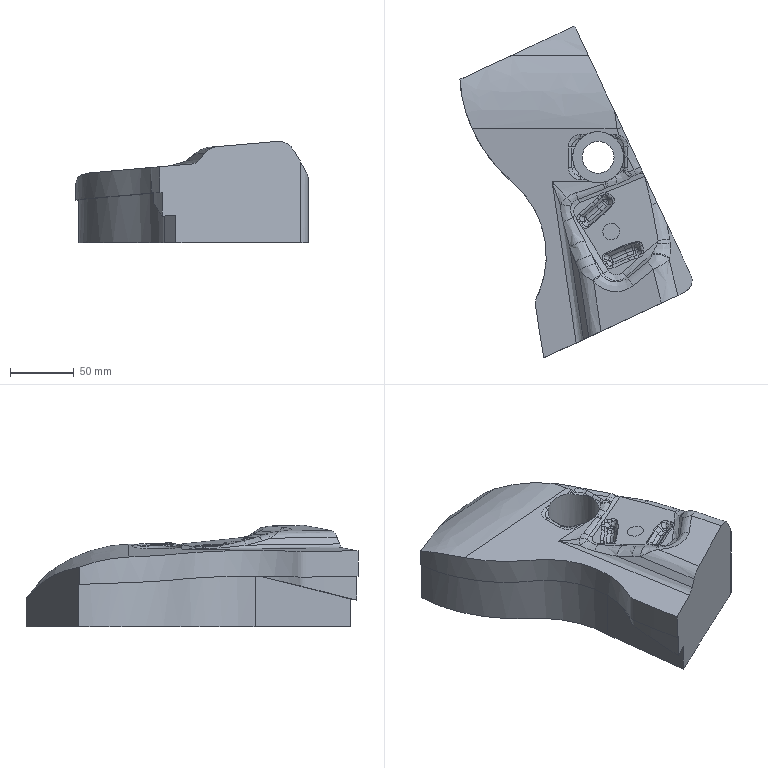Part | NX | features solid 2 | 1 solid | 166 faces | box 181.501 x 259.516 x 79.281 mm | volume 1341159 mm3 | spline 156 | plane 7 | cylinder 3 | commonest cylinder face diameters 20 x1 25 x1 40 x1